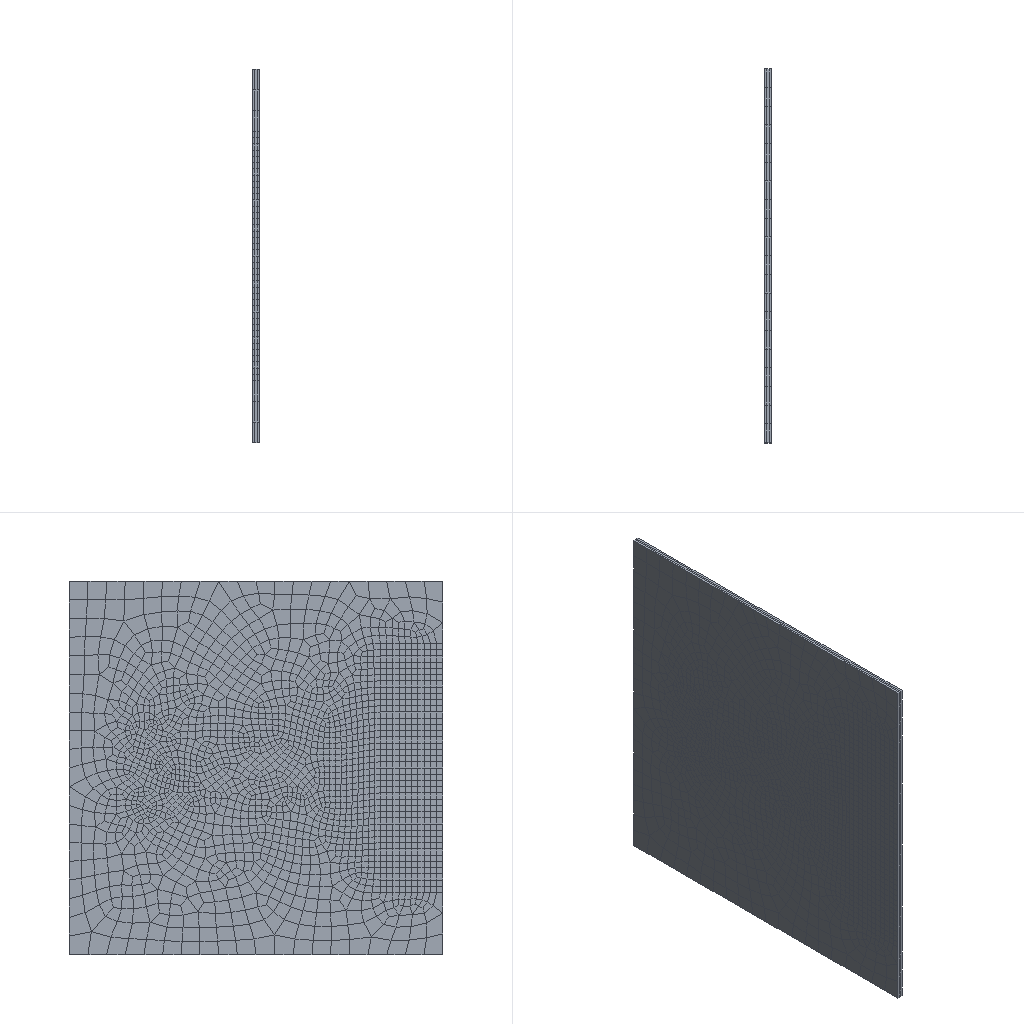Simulation study | abaqus
Set-up summary:
category,name,step,type,value,unit,region
solver,abaqus
solver,version,,,Abaqus/Standard 2020
units,not stated in the deck,,not stated
analysis,deck,,modal,modal
load_step,Step-1,Step-1,modal,nlgeom=False
contact,interactions,,,general=0 pairs=0 ties=0
load_step,requested,,,1
mesh,nodes,,,8868
mesh,elements,,,6489
element_type,C3D8R,,solid,6489
load,load commands in deck,,count,0
bc,support commands in deck,,count,4
material,MATERIAL-1,,in results
check,setup vs results,,match,"per instance, exact: element labels, types and connectivity; labels of the nodes the elements use; coordinates of those nodes at SINGLE_PRECISION in 1 of 1 instance(s)"
Abaqus input file, long lists of numbers shortened:
*Heading
** Job name: Job-1 Model name: Model-1
** Generated by: Abaqus/CAE 2020
*Preprint, echo=NO, model=NO, history=NO, contact=NO
**
** PARTS
**
*Part, name=work-8
*Node
      1,  -5.927,   40.385,        -100.
      2,  -5.927,   15.385,        -100.
** (8866 more lines like these left out)
*Element, type=C3D8R
  1,  199,  977, 4923,  821,    1,   25,  509,  110
  2,  977,  978, 4924, 4923,   25,   26,  510,  509
** (6487 more lines like these left out)
*Nset, nset=Set-3, generate
    1,  8868,     1
*Elset, elset=Set-3, generate
    1,  6489,     1
** Section: Section-1
*Solid Section, elset=Set-3, material=Material-1
,
*End Part
**
**
** ASSEMBLY
**
*Assembly, name=Assembly
**
*Instance, name=work-8-1, part=work-8
*End Instance
**
*Node
      1, -0.927,   255.385,           0.
*Nset, nset=Set-1, instance=work-8-1
   2,   3,   5,   6,  29,  30,  31,  32,  33,  34,  35,  36,  37,  38,  39,  40
  41,  42,  43,  44,  45,  46,  47,  48,  49,  50,  51,  52,  53,  54,  55,  56
** (9 more lines like these left out)
*Elset, elset=Set-1, instance=work-8-1, generate
   5,  600,    5
*Nset, nset=Set-2, instance=work-8-1
    1,    4,    7,    8,    9,   10,   11,   12,   72,   73,   74,   75,   76,   77,   78,   79
   80,   81,   82,   83,   84,   85,   86,   87,   88,   89,   90,   91,   92,   93,   94,   95
** (29 more lines like these left out)
*Elset, elset=Set-2, instance=work-8-1
  601,  602,  603,  604,  605,  606,  607,  608,  609,  610,  611,  612,  613,  614,  615,  616
  617,  618,  619,  620,  621,  622,  623,  624,  625,  626,  627,  628,  629,  630,  631,  632
** (23 more lines like these left out)
*Nset, nset=m_Set-3
 1,
*Elset, elset=_s_Surf-1_S1, internal, instance=work-8-1, generate
 6312,  6360,     1
*Elset, elset=_s_Surf-1_S2, internal, instance=work-8-1, generate
 6361,  6403,     1
*Surface, type=ELEMENT, name=s_Surf-1
_s_Surf-1_S1, S1
_s_Surf-1_S2, S2
** Constraint: Constraint-1
*Coupling, constraint name=Constraint-1, ref node=m_Set-3, surface=s_Surf-1
*Kinematic
*Spring, elset=Springs/Dashpots-1-spring
1
250.
*Dashpot, elset=Springs/Dashpots-1-dashpot
1
0.08
*Element, type=Spring1, elset=Springs/Dashpots-1-spring
1, 1
*Element, type=Dashpot1, elset=Springs/Dashpots-1-dashpot
2, 1
*End Assembly
**
** MATERIALS
**
*Material, name=Material-1
*Density
 2.75e-09,
*Elastic
68900., 0.33
** ----------------------------------------------------------------
**
** STEP: Step-1
**
*Step, name=Step-1, nlgeom=NO, perturbation
*Frequency, eigensolver=Lanczos, sim, acoustic coupling=on, normalization=mass
10, , , , ,
**
** BOUNDARY CONDITIONS
**
** Name: BC-1 Type: 位移/转角
*Boundary
Set-1, 2, 2
Set-1, 3, 3
** Name: BC-2 Type: 位移/转角
*Boundary
Set-2, 1, 1
Set-2, 3, 3
**
** OUTPUT REQUESTS
**
*Restart, write, frequency=0
**
** FIELD OUTPUT: F-Output-1
**
*Output, field, variable=PRESELECT
*End Step
Results summary:
result,step,,partial,increments=0 time=0.0/1e-36
result,analysis,,,modal
result,last_loadstep,,,1
result,analysis steps,,count,1
result,primary field,,,U